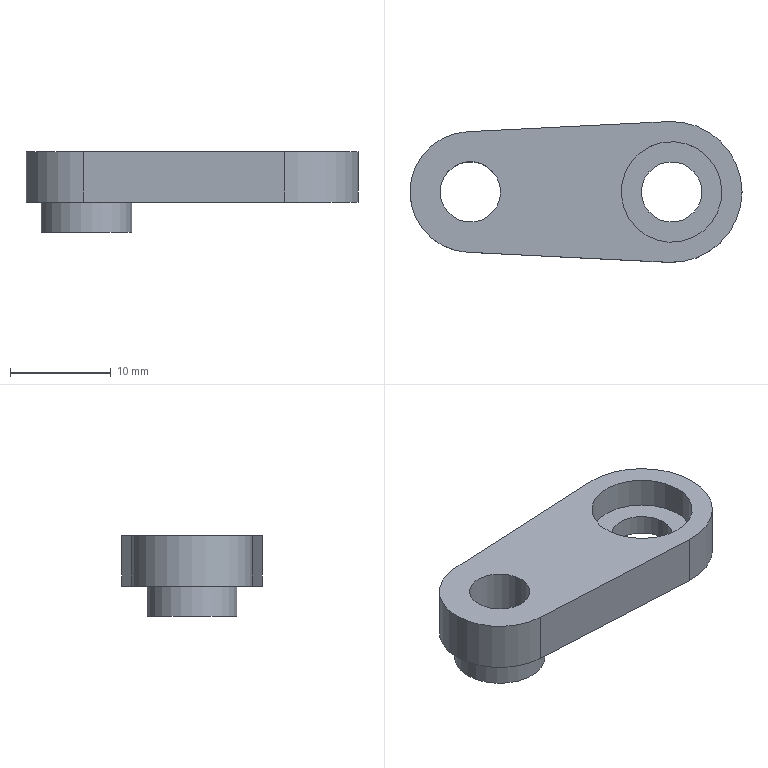Part | NX | features BREP 1, DATUM_CSYS 1 | 1 solid | 12 faces | box 33 x 14 x 8 mm | volume 1642 mm3 | plane 6 | cylinder 6 | commonest cylinder face diameters 6 x2 9 x1 10 x1 12 x1 14 x1
STEP:
#1=CARTESIAN_POINT('',(4.5,0.,0.));
#2=VERTEX_POINT('',#1);
#3=CARTESIAN_POINT('',(0.,0.,0.));
#4=DIRECTION('',(0.,0.,1.));
#5=DIRECTION('',(1.,0.,0.));
#6=AXIS2_PLACEMENT_3D('',#3,#4,#5);
#7=CIRCLE('',#6,4.5);
#8=EDGE_CURVE('',#2,#2,#7,.T.);
#9=ORIENTED_EDGE('',*,*,#8,.F.);
#10=EDGE_LOOP('',(#9));
#11=FACE_BOUND('',#10,.T.);
#12=CARTESIAN_POINT('',(3.,0.,0.));
#13=VERTEX_POINT('',#12);
#14=CARTESIAN_POINT('',(0.,0.,0.));
#15=DIRECTION('',(0.,0.,-1.));
#16=DIRECTION('',(1.,0.,0.));
#17=AXIS2_PLACEMENT_3D('',#14,#15,#16);
#18=CIRCLE('',#17,3.);
#19=EDGE_CURVE('',#13,#13,#18,.T.);
#20=ORIENTED_EDGE('',*,*,#19,.F.);
#21=EDGE_LOOP('',(#20));
#22=FACE_BOUND('',#21,.T.);
#23=CARTESIAN_POINT('',(10.5,9.141,0.));
#24=DIRECTION('',(0.,0.,1.));
#25=DIRECTION('',(-1.,0.,0.));
#26=AXIS2_PLACEMENT_3D('',#23,#24,#25);
#27=PLANE('',#26);
#28=ADVANCED_FACE('',(#11,#22),#27,.F.);
#29=CARTESIAN_POINT('',(-0.3,5.992,8.));
#30=VERTEX_POINT('',#29);
#31=CARTESIAN_POINT('',(-0.3,-5.992,8.));
#32=VERTEX_POINT('',#31);
#33=CARTESIAN_POINT('',(0.,0.,8.));
#34=DIRECTION('',(0.,0.,1.));
#35=DIRECTION('',(-0.05,0.9987,0.));
#36=AXIS2_PLACEMENT_3D('',#33,#34,#35);
#37=CIRCLE('',#36,6.);
#38=EDGE_CURVE('',#30,#32,#37,.T.);
#39=ORIENTED_EDGE('',*,*,#38,.T.);
#40=CARTESIAN_POINT('',(19.65,-6.991,8.));
#41=VERTEX_POINT('',#40);
#42=CARTESIAN_POINT('',(-0.3,-5.992,8.));
#43=DIRECTION('',(0.9987,-0.05,0.));
#44=VECTOR('',#43,1000.);
#45=LINE('',#42,#44);
#46=EDGE_CURVE('',#32,#41,#45,.T.);
#47=ORIENTED_EDGE('',*,*,#46,.T.);
#48=CARTESIAN_POINT('',(19.65,6.991,8.));
#49=VERTEX_POINT('',#48);
#50=CARTESIAN_POINT('',(20.,0.,8.));
#51=DIRECTION('',(0.,0.,1.));
#52=DIRECTION('',(-0.05,-0.9987,0.));
#53=AXIS2_PLACEMENT_3D('',#50,#51,#52);
#54=CIRCLE('',#53,7.);
#55=EDGE_CURVE('',#41,#49,#54,.T.);
#56=ORIENTED_EDGE('',*,*,#55,.T.);
#57=CARTESIAN_POINT('',(19.65,6.991,8.));
#58=DIRECTION('',(-0.9987,-0.05,0.));
#59=VECTOR('',#58,1000.);
#60=LINE('',#57,#59);
#61=EDGE_CURVE('',#49,#30,#60,.T.);
#62=ORIENTED_EDGE('',*,*,#61,.T.);
#63=EDGE_LOOP('',(#39,#47,#56,#62));
#64=FACE_BOUND('',#63,.T.);
#65=CARTESIAN_POINT('',(19.75,-4.994,8.));
#66=VERTEX_POINT('',#65);
#67=CARTESIAN_POINT('',(20.,0.,8.));
#68=DIRECTION('',(0.,0.,-1.));
#69=DIRECTION('',(-0.05,-0.9987,0.));
#70=AXIS2_PLACEMENT_3D('',#67,#68,#69);
#71=CIRCLE('',#70,5.);
#72=EDGE_CURVE('',#66,#66,#71,.T.);
#73=ORIENTED_EDGE('',*,*,#72,.T.);
#74=EDGE_LOOP('',(#73));
#75=FACE_BOUND('',#74,.T.);
#76=CARTESIAN_POINT('',(3.,0.,8.));
#77=VERTEX_POINT('',#76);
#78=CARTESIAN_POINT('',(0.,0.,8.));
#79=DIRECTION('',(0.,0.,-1.));
#80=DIRECTION('',(1.,0.,0.));
#81=AXIS2_PLACEMENT_3D('',#78,#79,#80);
#82=CIRCLE('',#81,3.);
#83=EDGE_CURVE('',#77,#77,#82,.T.);
#84=ORIENTED_EDGE('',*,*,#83,.T.);
#85=EDGE_LOOP('',(#84));
#86=FACE_BOUND('',#85,.T.);
#87=CARTESIAN_POINT('',(10.5,9.141,8.));
#88=DIRECTION('',(0.,0.,1.));
#89=DIRECTION('',(-1.,0.,0.));
#90=AXIS2_PLACEMENT_3D('',#87,#88,#89);
#91=PLANE('',#90);
#92=ADVANCED_FACE('',(#64,#75,#86),#91,.T.);
#93=CARTESIAN_POINT('',(19.65,-6.991,3.));
#94=VERTEX_POINT('',#93);
#95=CARTESIAN_POINT('',(19.65,-6.991,3.));
#96=DIRECTION('',(0.,0.,1.));
#97=VECTOR('',#96,1000.);
#98=LINE('',#95,#97);
#99=EDGE_CURVE('',#94,#41,#98,.T.);
#100=ORIENTED_EDGE('',*,*,#99,.T.);
#101=ORIENTED_EDGE('',*,*,#46,.F.);
#102=CARTESIAN_POINT('',(-0.3,-5.992,3.));
#103=VERTEX_POINT('',#102);
#104=CARTESIAN_POINT('',(-0.3,-5.992,3.));
#105=DIRECTION('',(0.,0.,1.));
#106=VECTOR('',#105,1000.);
#107=LINE('',#104,#106);
#108=EDGE_CURVE('',#103,#32,#107,.T.);
#109=ORIENTED_EDGE('',*,*,#108,.F.);
#110=CARTESIAN_POINT('',(19.65,-6.991,3.));
#111=DIRECTION('',(-0.9987,0.05,0.));
#112=VECTOR('',#111,1000.);
#113=LINE('',#110,#112);
#114=EDGE_CURVE('',#94,#103,#113,.T.);
#115=ORIENTED_EDGE('',*,*,#114,.F.);
#116=EDGE_LOOP('',(#100,#101,#109,#115));
#117=FACE_BOUND('',#116,.T.);
#118=CARTESIAN_POINT('',(9.675,-6.492,4.));
#119=DIRECTION('',(-0.05,-0.9987,0.));
#120=DIRECTION('',(-0.9987,0.05,0.));
#121=AXIS2_PLACEMENT_3D('',#118,#119,#120);
#122=PLANE('',#121);
#123=ADVANCED_FACE('',(#117),#122,.T.);
#124=ORIENTED_EDGE('',*,*,#55,.F.);
#125=ORIENTED_EDGE('',*,*,#99,.F.);
#126=CARTESIAN_POINT('',(19.65,6.991,3.));
#127=VERTEX_POINT('',#126);
#128=CARTESIAN_POINT('',(20.,0.,3.));
#129=DIRECTION('',(0.,0.,-1.));
#130=DIRECTION('',(-0.05,0.9987,0.));
#131=AXIS2_PLACEMENT_3D('',#128,#129,#130);
#132=CIRCLE('',#131,7.);
#133=EDGE_CURVE('',#127,#94,#132,.T.);
#134=ORIENTED_EDGE('',*,*,#133,.F.);
#135=CARTESIAN_POINT('',(19.65,6.991,3.));
#136=DIRECTION('',(0.,0.,1.));
#137=VECTOR('',#136,1000.);
#138=LINE('',#135,#137);
#139=EDGE_CURVE('',#127,#49,#138,.T.);
#140=ORIENTED_EDGE('',*,*,#139,.T.);
#141=EDGE_LOOP('',(#124,#125,#134,#140));
#142=FACE_BOUND('',#141,.T.);
#143=CARTESIAN_POINT('',(20.,0.,0.));
#144=DIRECTION('',(0.,0.,1.));
#145=DIRECTION('',(0.05,0.9987,0.));
#146=AXIS2_PLACEMENT_3D('',#143,#144,#145);
#147=CYLINDRICAL_SURFACE('',#146,7.);
#148=ADVANCED_FACE('',(#142),#147,.T.);
#149=ORIENTED_EDGE('',*,*,#61,.F.);
#150=ORIENTED_EDGE('',*,*,#139,.F.);
#151=CARTESIAN_POINT('',(-0.3,5.992,3.));
#152=VERTEX_POINT('',#151);
#153=CARTESIAN_POINT('',(19.65,6.991,3.));
#154=DIRECTION('',(-0.9987,-0.05,0.));
#155=VECTOR('',#154,1000.);
#156=LINE('',#153,#155);
#157=EDGE_CURVE('',#127,#152,#156,.T.);
#158=ORIENTED_EDGE('',*,*,#157,.T.);
#159=CARTESIAN_POINT('',(-0.3,5.992,3.));
#160=DIRECTION('',(0.,0.,1.));
#161=VECTOR('',#160,1000.);
#162=LINE('',#159,#161);
#163=EDGE_CURVE('',#152,#30,#162,.T.);
#164=ORIENTED_EDGE('',*,*,#163,.T.);
#165=EDGE_LOOP('',(#149,#150,#158,#164));
#166=FACE_BOUND('',#165,.T.);
#167=CARTESIAN_POINT('',(9.675,6.492,4.));
#168=DIRECTION('',(-0.05,0.9987,0.));
#169=DIRECTION('',(0.9987,0.05,0.));
#170=AXIS2_PLACEMENT_3D('',#167,#168,#169);
#171=PLANE('',#170);
#172=ADVANCED_FACE('',(#166),#171,.T.);
#173=CARTESIAN_POINT('',(19.75,-4.994,5.));
#174=VERTEX_POINT('',#173);
#175=CARTESIAN_POINT('',(19.75,-4.994,8.));
#176=DIRECTION('',(0.,0.,-1.));
#177=VECTOR('',#176,1000.);
#178=LINE('',#175,#177);
#179=EDGE_CURVE('',#66,#174,#178,.T.);
#180=ORIENTED_EDGE('',*,*,#179,.T.);
#181=CARTESIAN_POINT('',(20.,0.,5.));
#182=DIRECTION('',(0.,0.,-1.));
#183=DIRECTION('',(-0.05,-0.9987,0.));
#184=AXIS2_PLACEMENT_3D('',#181,#182,#183);
#185=CIRCLE('',#184,5.);
#186=EDGE_CURVE('',#174,#174,#185,.T.);
#187=ORIENTED_EDGE('',*,*,#186,.T.);
#188=ORIENTED_EDGE('',*,*,#179,.F.);
#189=ORIENTED_EDGE('',*,*,#72,.F.);
#190=EDGE_LOOP('',(#180,#187,#188,#189));
#191=FACE_BOUND('',#190,.T.);
#192=CARTESIAN_POINT('',(20.,0.,8.));
#193=DIRECTION('',(0.,0.,-1.));
#194=DIRECTION('',(0.05,0.9987,0.));
#195=AXIS2_PLACEMENT_3D('',#192,#193,#194);
#196=CYLINDRICAL_SURFACE('',#195,5.);
#197=ADVANCED_FACE('',(#191),#196,.F.);
#198=ORIENTED_EDGE('',*,*,#186,.F.);
#199=EDGE_LOOP('',(#198));
#200=FACE_BOUND('',#199,.T.);
#201=CARTESIAN_POINT('',(23.,0.,5.));
#202=VERTEX_POINT('',#201);
#203=CARTESIAN_POINT('',(20.,0.,5.));
#204=DIRECTION('',(0.,0.,-1.));
#205=DIRECTION('',(1.,0.,0.));
#206=AXIS2_PLACEMENT_3D('',#203,#204,#205);
#207=CIRCLE('',#206,3.);
#208=EDGE_CURVE('',#202,#202,#207,.T.);
#209=ORIENTED_EDGE('',*,*,#208,.T.);
#210=EDGE_LOOP('',(#209));
#211=FACE_BOUND('',#210,.T.);
#212=CARTESIAN_POINT('',(20.,0.,5.));
#213=DIRECTION('',(0.,0.,-1.));
#214=DIRECTION('',(0.05,0.9987,0.));
#215=AXIS2_PLACEMENT_3D('',#212,#213,#214);
#216=PLANE('',#215);
#217=ADVANCED_FACE('',(#200,#211),#216,.F.);
#218=CARTESIAN_POINT('',(23.,0.,3.));
#219=VERTEX_POINT('',#218);
#220=CARTESIAN_POINT('',(23.,0.,5.));
#221=DIRECTION('',(0.,0.,-1.));
#222=VECTOR('',#221,1000.);
#223=LINE('',#220,#222);
#224=EDGE_CURVE('',#202,#219,#223,.T.);
#225=ORIENTED_EDGE('',*,*,#224,.T.);
#226=CARTESIAN_POINT('',(20.,0.,3.));
#227=DIRECTION('',(0.,0.,1.));
#228=DIRECTION('',(1.,0.,0.));
#229=AXIS2_PLACEMENT_3D('',#226,#227,#228);
#230=CIRCLE('',#229,3.);
#231=EDGE_CURVE('',#219,#219,#230,.T.);
#232=ORIENTED_EDGE('',*,*,#231,.F.);
#233=ORIENTED_EDGE('',*,*,#224,.F.);
#234=ORIENTED_EDGE('',*,*,#208,.F.);
#235=EDGE_LOOP('',(#225,#232,#233,#234));
#236=FACE_BOUND('',#235,.T.);
#237=CARTESIAN_POINT('',(20.,0.,5.));
#238=DIRECTION('',(0.,0.,-1.));
#239=DIRECTION('',(-1.,0.,0.));
#240=AXIS2_PLACEMENT_3D('',#237,#238,#239);
#241=CYLINDRICAL_SURFACE('',#240,3.);
#242=ADVANCED_FACE('',(#236),#241,.F.);
#243=CARTESIAN_POINT('',(3.,0.,8.));
#244=DIRECTION('',(0.,0.,-1.));
#245=VECTOR('',#244,1000.);
#246=LINE('',#243,#245);
#247=EDGE_CURVE('',#77,#13,#246,.T.);
#248=ORIENTED_EDGE('',*,*,#247,.T.);
#249=ORIENTED_EDGE('',*,*,#19,.T.);
#250=ORIENTED_EDGE('',*,*,#247,.F.);
#251=ORIENTED_EDGE('',*,*,#83,.F.);
#252=EDGE_LOOP('',(#248,#249,#250,#251));
#253=FACE_BOUND('',#252,.T.);
#254=CARTESIAN_POINT('',(0.,0.,8.));
#255=DIRECTION('',(0.,0.,-1.));
#256=DIRECTION('',(-1.,0.,0.));
#257=AXIS2_PLACEMENT_3D('',#254,#255,#256);
#258=CYLINDRICAL_SURFACE('',#257,3.);
#259=ADVANCED_FACE('',(#253),#258,.F.);
#260=ORIENTED_EDGE('',*,*,#108,.T.);
#261=ORIENTED_EDGE('',*,*,#38,.F.);
#262=ORIENTED_EDGE('',*,*,#163,.F.);
#263=CARTESIAN_POINT('',(0.,0.,3.));
#264=DIRECTION('',(0.,0.,-1.));
#265=DIRECTION('',(-0.05,-0.9987,0.));
#266=AXIS2_PLACEMENT_3D('',#263,#264,#265);
#267=CIRCLE('',#266,6.);
#268=EDGE_CURVE('',#103,#152,#267,.T.);
#269=ORIENTED_EDGE('',*,*,#268,.F.);
#270=EDGE_LOOP('',(#260,#261,#262,#269));
#271=FACE_BOUND('',#270,.T.);
#272=CARTESIAN_POINT('',(0.,0.,0.));
#273=DIRECTION('',(0.,0.,1.));
#274=DIRECTION('',(0.05,-0.9987,0.));
#275=AXIS2_PLACEMENT_3D('',#272,#273,#274);
#276=CYLINDRICAL_SURFACE('',#275,6.);
#277=ADVANCED_FACE('',(#271),#276,.T.);
#278=ORIENTED_EDGE('',*,*,#268,.T.);
#279=ORIENTED_EDGE('',*,*,#157,.F.);
#280=ORIENTED_EDGE('',*,*,#133,.T.);
#281=ORIENTED_EDGE('',*,*,#114,.T.);
#282=EDGE_LOOP('',(#278,#279,#280,#281));
#283=FACE_BOUND('',#282,.T.);
#284=ORIENTED_EDGE('',*,*,#231,.T.);
#285=EDGE_LOOP('',(#284));
#286=FACE_BOUND('',#285,.T.);
#287=CARTESIAN_POINT('',(4.5,0.,3.));
#288=VERTEX_POINT('',#287);
#289=CARTESIAN_POINT('',(0.,0.,3.));
#290=DIRECTION('',(0.,0.,1.));
#291=DIRECTION('',(1.,0.,0.));
#292=AXIS2_PLACEMENT_3D('',#289,#290,#291);
#293=CIRCLE('',#292,4.5);
#294=EDGE_CURVE('',#288,#288,#293,.T.);
#295=ORIENTED_EDGE('',*,*,#294,.T.);
#296=EDGE_LOOP('',(#295));
#297=FACE_BOUND('',#296,.T.);
#298=CARTESIAN_POINT('',(-7.067,0.,3.));
#299=DIRECTION('',(0.,0.,-1.));
#300=DIRECTION('',(-1.,0.,0.));
#301=AXIS2_PLACEMENT_3D('',#298,#299,#300);
#302=PLANE('',#301);
#303=ADVANCED_FACE('',(#283,#286,#297),#302,.T.);
#304=ORIENTED_EDGE('',*,*,#8,.T.);
#305=CARTESIAN_POINT('',(4.5,0.,0.));
#306=DIRECTION('',(0.,0.,1.));
#307=VECTOR('',#306,1000.);
#308=LINE('',#305,#307);
#309=EDGE_CURVE('',#2,#288,#308,.T.);
#310=ORIENTED_EDGE('',*,*,#309,.T.);
#311=ORIENTED_EDGE('',*,*,#294,.F.);
#312=ORIENTED_EDGE('',*,*,#309,.F.);
#313=EDGE_LOOP('',(#304,#310,#311,#312));
#314=FACE_BOUND('',#313,.T.);
#315=CARTESIAN_POINT('',(0.,0.,0.));
#316=DIRECTION('',(0.,0.,1.));
#317=DIRECTION('',(-1.,0.,0.));
#318=AXIS2_PLACEMENT_3D('',#315,#316,#317);
#319=CYLINDRICAL_SURFACE('',#318,4.5);
#320=ADVANCED_FACE('',(#314),#319,.T.);
#321=CLOSED_SHELL('',(#28,#92,#123,#148,#172,#197,#217,#242,#259,#277,#303,#320));
#322=MANIFOLD_SOLID_BREP('',#321);
#323=(LENGTH_UNIT()NAMED_UNIT(*)SI_UNIT(.MILLI.,.METRE.));
#324=UNCERTAINTY_MEASURE_WITH_UNIT(LENGTH_MEASURE(0.00001),#323,'','');
#325=(NAMED_UNIT(*)PLANE_ANGLE_UNIT()SI_UNIT($,.RADIAN.));
#326=(NAMED_UNIT(*)SI_UNIT($,.STERADIAN.)SOLID_ANGLE_UNIT());
#327=(GEOMETRIC_REPRESENTATION_CONTEXT(3)GLOBAL_UNCERTAINTY_ASSIGNED_CONTEXT((#324))GLOBAL_UNIT_ASSIGNED_CONTEXT((#323,#325,#326))REPRESENTATION_CONTEXT('',''));
#328=ADVANCED_BREP_SHAPE_REPRESENTATION('',(#322),#327);